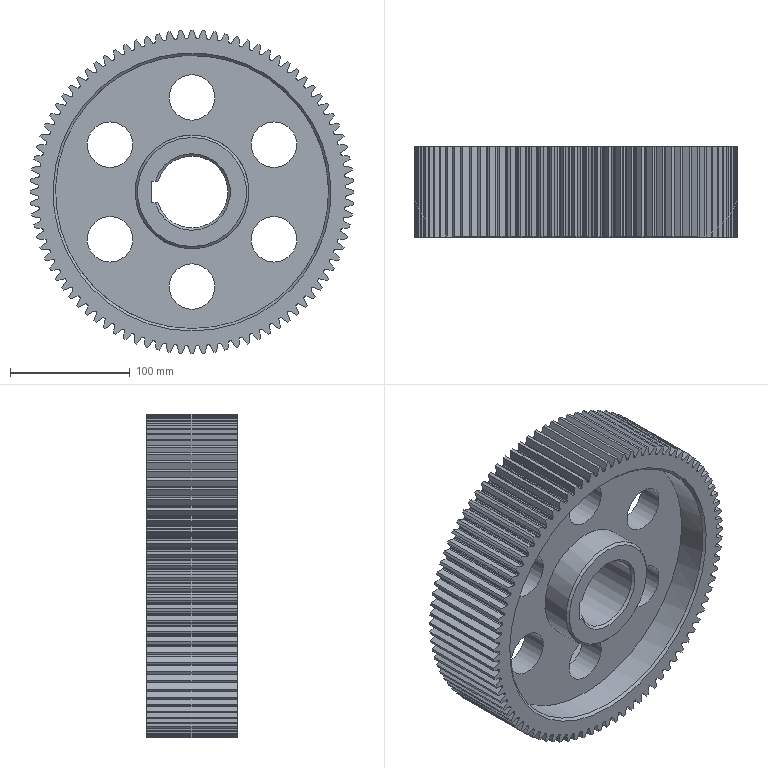Part | NX | features BREP 88, META 88, DATUM_CSYS 10, EXTRUDE 9, SKETCH 9, EXTRACT_DATUM_AXIS 8, EXTRACT_STRING 8, EXTRACT_DATUM_PLANE 6, Instance Feature 6, EXTRACT_FACE 2, CHAMFER 1, CYLINDER 1, FSET 1, Mirror Feature 1, Pattern Feature 1 | 1 solid | 554 faces | box 270 x 75.43 x 270 mm | volume 1925103 mm3 | spline 440 | cylinder 99 | plane 9 | cone 6 | commonest cylinder face diameters 256.5 x88 38 x6 95 x2 228 x2 60 x1